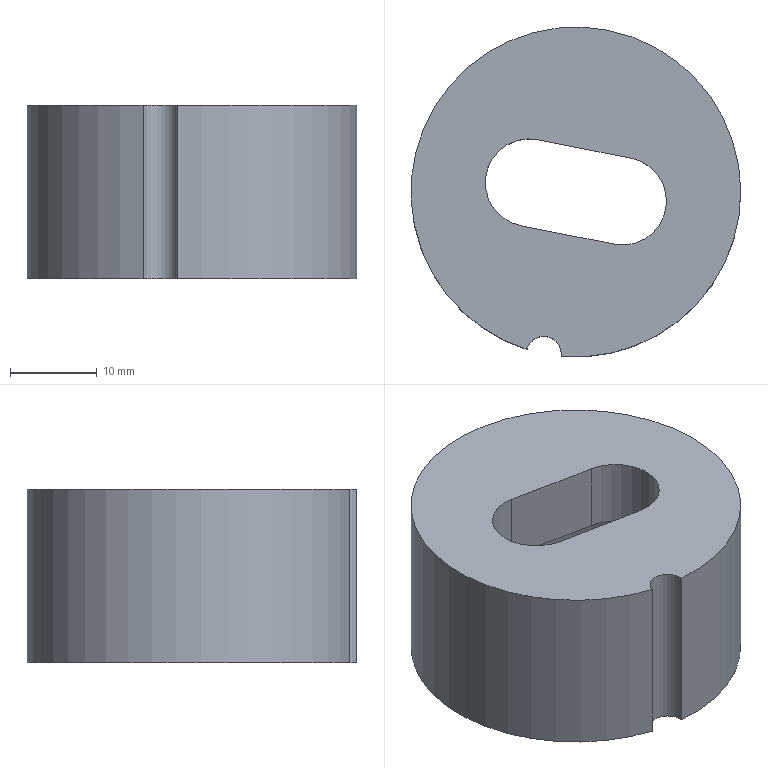Part | NX | features solid 2 | 1 solid | 10 faces | box 38 x 38 x 20 mm | volume 14361 mm3 | cylinder 5 | plane 5 | commonest cylinder face diameters 10.1 x2 4 x1 26.6 x1 38 x1
STEP:
#1=CARTESIAN_POINT('',(-746.596,310.341,19.));
#2=VERTEX_POINT('',#1);
#3=CARTESIAN_POINT('',(-746.596,310.341,39.));
#4=VERTEX_POINT('',#3);
#5=CARTESIAN_POINT('',(-746.596,310.341,29.));
#6=DIRECTION('',(0.,0.,1.));
#7=VECTOR('',#6,1000.);
#8=LINE('',#5,#7);
#9=EDGE_CURVE('',#2,#4,#8,.T.);
#10=ORIENTED_EDGE('',*,*,#9,.F.);
#11=CARTESIAN_POINT('',(-750.515,311.117,19.));
#12=VERTEX_POINT('',#11);
#13=CARTESIAN_POINT('',(-744.885,329.264,19.));
#14=DIRECTION('',(0.,0.,1.));
#15=DIRECTION('',(-0.1943,-0.9809,0.));
#16=AXIS2_PLACEMENT_3D('',#13,#14,#15);
#17=CIRCLE('',#16,19.);
#18=EDGE_CURVE('',#2,#12,#17,.T.);
#19=ORIENTED_EDGE('',*,*,#18,.T.);
#20=CARTESIAN_POINT('',(-750.515,311.117,39.));
#21=VERTEX_POINT('',#20);
#22=CARTESIAN_POINT('',(-750.515,311.117,29.));
#23=DIRECTION('',(0.,0.,1.));
#24=VECTOR('',#23,1000.);
#25=LINE('',#22,#24);
#26=EDGE_CURVE('',#21,#12,#25,.F.);
#27=ORIENTED_EDGE('',*,*,#26,.F.);
#28=CARTESIAN_POINT('',(-744.885,329.264,39.));
#29=DIRECTION('',(0.,0.,1.));
#30=DIRECTION('',(-0.1943,-0.9809,0.));
#31=AXIS2_PLACEMENT_3D('',#28,#29,#30);
#32=CIRCLE('',#31,19.);
#33=EDGE_CURVE('',#4,#21,#32,.T.);
#34=ORIENTED_EDGE('',*,*,#33,.F.);
#35=EDGE_LOOP('',(#10,#19,#27,#34));
#36=FACE_BOUND('',#35,.T.);
#37=CARTESIAN_POINT('',(-744.885,329.264,19.));
#38=DIRECTION('',(0.,0.,1.));
#39=DIRECTION('',(-0.1943,-0.9809,0.));
#40=AXIS2_PLACEMENT_3D('',#37,#38,#39);
#41=CYLINDRICAL_SURFACE('',#40,19.);
#42=ADVANCED_FACE('',(#36),#41,.T.);
#43=CARTESIAN_POINT('',(-747.469,316.217,19.));
#44=VERTEX_POINT('',#43);
#45=CARTESIAN_POINT('',(-744.885,329.264,19.));
#46=DIRECTION('',(0.,0.,1.));
#47=DIRECTION('',(-0.1943,-0.9809,0.));
#48=AXIS2_PLACEMENT_3D('',#45,#46,#47);
#49=CIRCLE('',#48,13.3);
#50=EDGE_CURVE('',#44,#44,#49,.T.);
#51=ORIENTED_EDGE('',*,*,#50,.T.);
#52=EDGE_LOOP('',(#51));
#53=FACE_BOUND('',#52,.T.);
#54=ORIENTED_EDGE('',*,*,#18,.F.);
#55=CARTESIAN_POINT('',(-748.576,310.626,19.));
#56=DIRECTION('',(0.,0.,1.));
#57=DIRECTION('',(-0.1943,-0.9809,0.));
#58=AXIS2_PLACEMENT_3D('',#55,#56,#57);
#59=CIRCLE('',#58,2.);
#60=EDGE_CURVE('',#2,#12,#59,.T.);
#61=ORIENTED_EDGE('',*,*,#60,.T.);
#62=EDGE_LOOP('',(#54,#61));
#63=FACE_BOUND('',#62,.T.);
#64=CARTESIAN_POINT('',(-744.885,329.264,19.));
#65=DIRECTION('',(0.,0.,1.));
#66=DIRECTION('',(-0.1943,-0.9809,0.));
#67=AXIS2_PLACEMENT_3D('',#64,#65,#66);
#68=PLANE('',#67);
#69=ADVANCED_FACE('',(#53,#63),#68,.F.);
#70=CARTESIAN_POINT('',(-738.508,333.149,39.));
#71=VERTEX_POINT('',#70);
#72=CARTESIAN_POINT('',(-749.299,335.286,39.));
#73=VERTEX_POINT('',#72);
#74=CARTESIAN_POINT('',(-738.508,333.149,39.));
#75=DIRECTION('',(-0.9809,0.1943,0.));
#76=VECTOR('',#75,1000.);
#77=LINE('',#74,#76);
#78=EDGE_CURVE('',#71,#73,#77,.T.);
#79=ORIENTED_EDGE('',*,*,#78,.F.);
#80=CARTESIAN_POINT('',(-740.471,323.241,39.));
#81=VERTEX_POINT('',#80);
#82=CARTESIAN_POINT('',(-739.489,328.195,39.));
#83=DIRECTION('',(0.,0.,1.));
#84=DIRECTION('',(-0.1943,-0.9809,0.));
#85=AXIS2_PLACEMENT_3D('',#82,#83,#84);
#86=CIRCLE('',#85,5.05);
#87=EDGE_CURVE('',#81,#71,#86,.T.);
#88=ORIENTED_EDGE('',*,*,#87,.F.);
#89=CARTESIAN_POINT('',(-751.261,325.378,39.));
#90=VERTEX_POINT('',#89);
#91=CARTESIAN_POINT('',(-740.471,323.241,39.));
#92=DIRECTION('',(-0.9809,0.1943,0.));
#93=VECTOR('',#92,1000.);
#94=LINE('',#91,#93);
#95=EDGE_CURVE('',#81,#90,#94,.T.);
#96=ORIENTED_EDGE('',*,*,#95,.T.);
#97=CARTESIAN_POINT('',(-750.28,330.332,39.));
#98=DIRECTION('',(0.,0.,1.));
#99=DIRECTION('',(-0.1943,-0.9809,0.));
#100=AXIS2_PLACEMENT_3D('',#97,#98,#99);
#101=CIRCLE('',#100,5.05);
#102=EDGE_CURVE('',#73,#90,#101,.T.);
#103=ORIENTED_EDGE('',*,*,#102,.F.);
#104=EDGE_LOOP('',(#79,#88,#96,#103));
#105=FACE_BOUND('',#104,.T.);
#106=CARTESIAN_POINT('',(-748.576,310.626,39.));
#107=DIRECTION('',(0.,0.,1.));
#108=DIRECTION('',(-0.1943,-0.9809,0.));
#109=AXIS2_PLACEMENT_3D('',#106,#107,#108);
#110=CIRCLE('',#109,2.);
#111=EDGE_CURVE('',#4,#21,#110,.T.);
#112=ORIENTED_EDGE('',*,*,#111,.F.);
#113=ORIENTED_EDGE('',*,*,#33,.T.);
#114=EDGE_LOOP('',(#112,#113));
#115=FACE_BOUND('',#114,.T.);
#116=CARTESIAN_POINT('',(-744.885,329.264,39.));
#117=DIRECTION('',(0.,0.,1.));
#118=DIRECTION('',(-0.1943,-0.9809,0.));
#119=AXIS2_PLACEMENT_3D('',#116,#117,#118);
#120=PLANE('',#119);
#121=ADVANCED_FACE('',(#105,#115),#120,.T.);
#122=ORIENTED_EDGE('',*,*,#50,.F.);
#123=EDGE_LOOP('',(#122));
#124=FACE_BOUND('',#123,.T.);
#125=CARTESIAN_POINT('',(-747.469,316.217,31.));
#126=VERTEX_POINT('',#125);
#127=CARTESIAN_POINT('',(-744.885,329.264,31.));
#128=DIRECTION('',(0.,0.,1.));
#129=DIRECTION('',(-0.1943,-0.9809,0.));
#130=AXIS2_PLACEMENT_3D('',#127,#128,#129);
#131=CIRCLE('',#130,13.3);
#132=EDGE_CURVE('',#126,#126,#131,.T.);
#133=ORIENTED_EDGE('',*,*,#132,.T.);
#134=EDGE_LOOP('',(#133));
#135=FACE_BOUND('',#134,.T.);
#136=CARTESIAN_POINT('',(-744.885,329.264,19.));
#137=DIRECTION('',(0.,0.,1.));
#138=DIRECTION('',(-0.1943,-0.9809,0.));
#139=AXIS2_PLACEMENT_3D('',#136,#137,#138);
#140=CYLINDRICAL_SURFACE('',#139,13.3);
#141=ADVANCED_FACE('',(#124,#135),#140,.F.);
#142=CARTESIAN_POINT('',(-740.471,323.241,31.));
#143=VERTEX_POINT('',#142);
#144=CARTESIAN_POINT('',(-738.508,333.149,31.));
#145=VERTEX_POINT('',#144);
#146=CARTESIAN_POINT('',(-739.489,328.195,31.));
#147=DIRECTION('',(0.,0.,1.));
#148=DIRECTION('',(-0.1943,-0.9809,0.));
#149=AXIS2_PLACEMENT_3D('',#146,#147,#148);
#150=CIRCLE('',#149,5.05);
#151=EDGE_CURVE('',#143,#145,#150,.T.);
#152=ORIENTED_EDGE('',*,*,#151,.T.);
#153=CARTESIAN_POINT('',(-749.299,335.286,31.));
#154=VERTEX_POINT('',#153);
#155=CARTESIAN_POINT('',(-743.904,334.217,31.));
#156=DIRECTION('',(-0.9809,0.1943,0.));
#157=VECTOR('',#156,1000.);
#158=LINE('',#155,#157);
#159=EDGE_CURVE('',#145,#154,#158,.T.);
#160=ORIENTED_EDGE('',*,*,#159,.T.);
#161=CARTESIAN_POINT('',(-751.261,325.378,31.));
#162=VERTEX_POINT('',#161);
#163=CARTESIAN_POINT('',(-750.28,330.332,31.));
#164=DIRECTION('',(0.,0.,1.));
#165=DIRECTION('',(-0.1943,-0.9809,0.));
#166=AXIS2_PLACEMENT_3D('',#163,#164,#165);
#167=CIRCLE('',#166,5.05);
#168=EDGE_CURVE('',#154,#162,#167,.T.);
#169=ORIENTED_EDGE('',*,*,#168,.T.);
#170=CARTESIAN_POINT('',(-745.866,324.31,31.));
#171=DIRECTION('',(-0.9809,0.1943,0.));
#172=VECTOR('',#171,1000.);
#173=LINE('',#170,#172);
#174=EDGE_CURVE('',#143,#162,#173,.T.);
#175=ORIENTED_EDGE('',*,*,#174,.F.);
#176=EDGE_LOOP('',(#152,#160,#169,#175));
#177=FACE_BOUND('',#176,.T.);
#178=ORIENTED_EDGE('',*,*,#132,.F.);
#179=EDGE_LOOP('',(#178));
#180=FACE_BOUND('',#179,.T.);
#181=CARTESIAN_POINT('',(-744.885,329.264,31.));
#182=DIRECTION('',(0.,0.,1.));
#183=DIRECTION('',(-0.1943,-0.9809,0.));
#184=AXIS2_PLACEMENT_3D('',#181,#182,#183);
#185=PLANE('',#184);
#186=ADVANCED_FACE('',(#177,#180),#185,.F.);
#187=ORIENTED_EDGE('',*,*,#9,.T.);
#188=ORIENTED_EDGE('',*,*,#111,.T.);
#189=ORIENTED_EDGE('',*,*,#26,.T.);
#190=ORIENTED_EDGE('',*,*,#60,.F.);
#191=EDGE_LOOP('',(#187,#188,#189,#190));
#192=FACE_BOUND('',#191,.T.);
#193=CARTESIAN_POINT('',(-748.576,310.626,19.));
#194=DIRECTION('',(0.,0.,1.));
#195=DIRECTION('',(-0.1943,-0.9809,0.));
#196=AXIS2_PLACEMENT_3D('',#193,#194,#195);
#197=CYLINDRICAL_SURFACE('',#196,2.);
#198=ADVANCED_FACE('',(#192),#197,.F.);
#199=CARTESIAN_POINT('',(-738.508,333.149,19.));
#200=DIRECTION('',(0.,0.,1.));
#201=VECTOR('',#200,1000.);
#202=LINE('',#199,#201);
#203=EDGE_CURVE('',#145,#71,#202,.T.);
#204=ORIENTED_EDGE('',*,*,#203,.T.);
#205=ORIENTED_EDGE('',*,*,#78,.T.);
#206=CARTESIAN_POINT('',(-749.299,335.286,19.));
#207=DIRECTION('',(0.,0.,1.));
#208=VECTOR('',#207,1000.);
#209=LINE('',#206,#208);
#210=EDGE_CURVE('',#154,#73,#209,.T.);
#211=ORIENTED_EDGE('',*,*,#210,.F.);
#212=ORIENTED_EDGE('',*,*,#159,.F.);
#213=EDGE_LOOP('',(#204,#205,#211,#212));
#214=FACE_BOUND('',#213,.T.);
#215=CARTESIAN_POINT('',(-738.508,333.149,19.));
#216=DIRECTION('',(0.1943,0.9809,0.));
#217=DIRECTION('',(0.,0.,1.));
#218=AXIS2_PLACEMENT_3D('',#215,#216,#217);
#219=PLANE('',#218);
#220=ADVANCED_FACE('',(#214),#219,.F.);
#221=ORIENTED_EDGE('',*,*,#210,.T.);
#222=ORIENTED_EDGE('',*,*,#102,.T.);
#223=CARTESIAN_POINT('',(-751.261,325.378,19.));
#224=DIRECTION('',(0.,0.,1.));
#225=VECTOR('',#224,1000.);
#226=LINE('',#223,#225);
#227=EDGE_CURVE('',#162,#90,#226,.T.);
#228=ORIENTED_EDGE('',*,*,#227,.F.);
#229=ORIENTED_EDGE('',*,*,#168,.F.);
#230=EDGE_LOOP('',(#221,#222,#228,#229));
#231=FACE_BOUND('',#230,.T.);
#232=CARTESIAN_POINT('',(-750.28,330.332,19.));
#233=DIRECTION('',(0.,0.,1.));
#234=DIRECTION('',(-0.1943,-0.9809,0.));
#235=AXIS2_PLACEMENT_3D('',#232,#233,#234);
#236=CYLINDRICAL_SURFACE('',#235,5.05);
#237=ADVANCED_FACE('',(#231),#236,.F.);
#238=ORIENTED_EDGE('',*,*,#174,.T.);
#239=ORIENTED_EDGE('',*,*,#227,.T.);
#240=ORIENTED_EDGE('',*,*,#95,.F.);
#241=CARTESIAN_POINT('',(-740.471,323.241,19.));
#242=DIRECTION('',(0.,0.,1.));
#243=VECTOR('',#242,1000.);
#244=LINE('',#241,#243);
#245=EDGE_CURVE('',#143,#81,#244,.T.);
#246=ORIENTED_EDGE('',*,*,#245,.F.);
#247=EDGE_LOOP('',(#238,#239,#240,#246));
#248=FACE_BOUND('',#247,.T.);
#249=CARTESIAN_POINT('',(-740.471,323.241,19.));
#250=DIRECTION('',(0.1943,0.9809,0.));
#251=DIRECTION('',(0.,0.,1.));
#252=AXIS2_PLACEMENT_3D('',#249,#250,#251);
#253=PLANE('',#252);
#254=ADVANCED_FACE('',(#248),#253,.T.);
#255=ORIENTED_EDGE('',*,*,#245,.T.);
#256=ORIENTED_EDGE('',*,*,#87,.T.);
#257=ORIENTED_EDGE('',*,*,#203,.F.);
#258=ORIENTED_EDGE('',*,*,#151,.F.);
#259=EDGE_LOOP('',(#255,#256,#257,#258));
#260=FACE_BOUND('',#259,.T.);
#261=CARTESIAN_POINT('',(-739.489,328.195,19.));
#262=DIRECTION('',(0.,0.,1.));
#263=DIRECTION('',(-0.1943,-0.9809,0.));
#264=AXIS2_PLACEMENT_3D('',#261,#262,#263);
#265=CYLINDRICAL_SURFACE('',#264,5.05);
#266=ADVANCED_FACE('',(#260),#265,.F.);
#267=CLOSED_SHELL('',(#42,#69,#121,#141,#186,#198,#220,#237,#254,#266));
#268=MANIFOLD_SOLID_BREP('',#267);
#269=(LENGTH_UNIT()NAMED_UNIT(*)SI_UNIT(.MILLI.,.METRE.));
#270=UNCERTAINTY_MEASURE_WITH_UNIT(LENGTH_MEASURE(0.00001),#269,'','');
#271=(NAMED_UNIT(*)PLANE_ANGLE_UNIT()SI_UNIT($,.RADIAN.));
#272=(NAMED_UNIT(*)SI_UNIT($,.STERADIAN.)SOLID_ANGLE_UNIT());
#273=(GEOMETRIC_REPRESENTATION_CONTEXT(3)GLOBAL_UNCERTAINTY_ASSIGNED_CONTEXT((#270))GLOBAL_UNIT_ASSIGNED_CONTEXT((#269,#271,#272))REPRESENTATION_CONTEXT('',''));
#274=ADVANCED_BREP_SHAPE_REPRESENTATION('',(#268),#273);